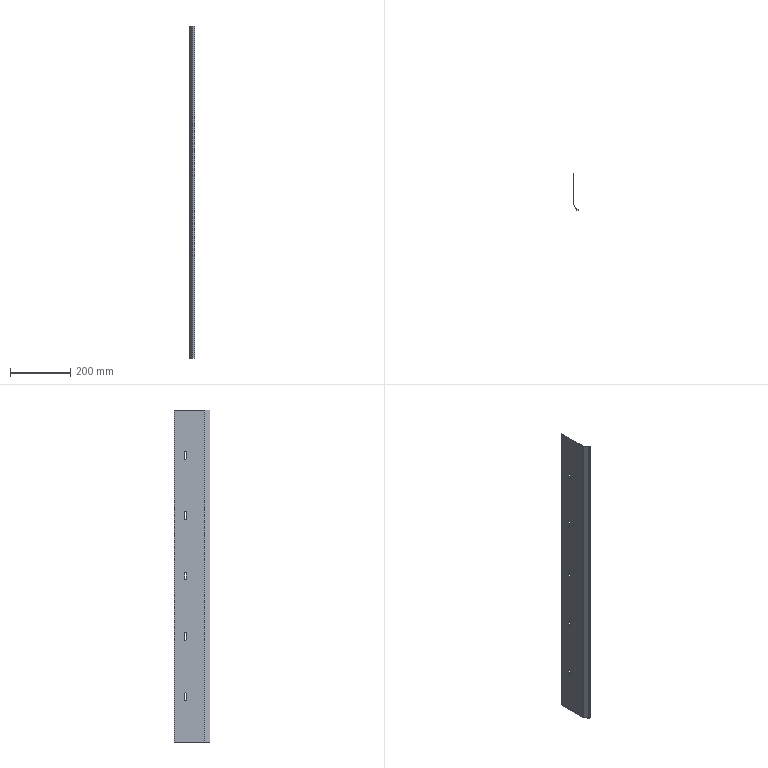Part | SolidWorks | features FlatPattern 1, ICE 1, SMBaseFlange 1, SheetMetal 1 | 1 solid | 47 faces | box 17 x 118.321 x 1100 mm | volume 138591 mm3 | plane 28 | cylinder 19 | commonest cylinder face diameters 6 x15 2 x2 4 x2
STEP:
#1=CARTESIAN_POINT('',(0.,-34.5,210.));
#2=VERTEX_POINT('',#1);
#3=CARTESIAN_POINT('',(0.,-37.5,213.));
#4=VERTEX_POINT('',#3);
#5=CARTESIAN_POINT('',(0.,-37.5,210.));
#6=DIRECTION('',(1.,0.,0.));
#7=DIRECTION('',(0.,1.,0.));
#8=AXIS2_PLACEMENT_3D('',#5,#6,#7);
#9=CIRCLE('',#8,3.);
#10=EDGE_CURVE('',#2,#4,#9,.T.);
#11=ORIENTED_EDGE('',*,*,#10,.T.);
#12=CARTESIAN_POINT('',(-1.,-37.5,213.));
#13=VERTEX_POINT('',#12);
#14=CARTESIAN_POINT('',(9.,-37.5,213.));
#15=DIRECTION('',(-1.,0.,0.));
#16=VECTOR('',#15,1000.);
#17=LINE('',#14,#16);
#18=EDGE_CURVE('',#4,#13,#17,.T.);
#19=ORIENTED_EDGE('',*,*,#18,.T.);
#20=CARTESIAN_POINT('',(-1.,-34.5,210.));
#21=VERTEX_POINT('',#20);
#22=CARTESIAN_POINT('',(-1.,-37.5,210.));
#23=DIRECTION('',(-1.,0.,0.));
#24=DIRECTION('',(0.,0.,-1.));
#25=AXIS2_PLACEMENT_3D('',#22,#23,#24);
#26=CIRCLE('',#25,3.);
#27=EDGE_CURVE('',#13,#21,#26,.T.);
#28=ORIENTED_EDGE('',*,*,#27,.T.);
#29=CARTESIAN_POINT('',(9.,-34.5,210.));
#30=DIRECTION('',(-1.,0.,0.));
#31=VECTOR('',#30,1000.);
#32=LINE('',#29,#31);
#33=EDGE_CURVE('',#2,#21,#32,.T.);
#34=ORIENTED_EDGE('',*,*,#33,.F.);
#35=EDGE_LOOP('',(#11,#19,#28,#34));
#36=FACE_OUTER_BOUND('',#35,.T.);
#37=CARTESIAN_POINT('',(9.,-37.5,210.));
#38=DIRECTION('',(-1.,0.,0.));
#39=DIRECTION('',(0.,0.,1.));
#40=AXIS2_PLACEMENT_3D('',#37,#38,#39);
#41=CYLINDRICAL_SURFACE('',#40,3.);
#42=ADVANCED_FACE('',(#36),#41,.F.);
#43=CARTESIAN_POINT('',(0.,-34.5,410.));
#44=VERTEX_POINT('',#43);
#45=CARTESIAN_POINT('',(0.,-37.5,413.));
#46=VERTEX_POINT('',#45);
#47=CARTESIAN_POINT('',(0.,-37.5,410.));
#48=DIRECTION('',(1.,0.,0.));
#49=DIRECTION('',(0.,1.,0.));
#50=AXIS2_PLACEMENT_3D('',#47,#48,#49);
#51=CIRCLE('',#50,3.);
#52=EDGE_CURVE('',#44,#46,#51,.T.);
#53=ORIENTED_EDGE('',*,*,#52,.T.);
#54=CARTESIAN_POINT('',(-1.,-37.5,413.));
#55=VERTEX_POINT('',#54);
#56=CARTESIAN_POINT('',(9.,-37.5,413.));
#57=DIRECTION('',(-1.,0.,0.));
#58=VECTOR('',#57,1000.);
#59=LINE('',#56,#58);
#60=EDGE_CURVE('',#46,#55,#59,.T.);
#61=ORIENTED_EDGE('',*,*,#60,.T.);
#62=CARTESIAN_POINT('',(-1.,-34.5,410.));
#63=VERTEX_POINT('',#62);
#64=CARTESIAN_POINT('',(-1.,-37.5,410.));
#65=DIRECTION('',(-1.,0.,0.));
#66=DIRECTION('',(0.,0.,-1.));
#67=AXIS2_PLACEMENT_3D('',#64,#65,#66);
#68=CIRCLE('',#67,3.);
#69=EDGE_CURVE('',#55,#63,#68,.T.);
#70=ORIENTED_EDGE('',*,*,#69,.T.);
#71=CARTESIAN_POINT('',(9.,-34.5,410.));
#72=DIRECTION('',(-1.,0.,0.));
#73=VECTOR('',#72,1000.);
#74=LINE('',#71,#73);
#75=EDGE_CURVE('',#44,#63,#74,.T.);
#76=ORIENTED_EDGE('',*,*,#75,.F.);
#77=EDGE_LOOP('',(#53,#61,#70,#76));
#78=FACE_OUTER_BOUND('',#77,.T.);
#79=CARTESIAN_POINT('',(9.,-37.5,410.));
#80=DIRECTION('',(-1.,0.,0.));
#81=DIRECTION('',(0.,0.,1.));
#82=AXIS2_PLACEMENT_3D('',#79,#80,#81);
#83=CYLINDRICAL_SURFACE('',#82,3.);
#84=ADVANCED_FACE('',(#78),#83,.F.);
#85=CARTESIAN_POINT('',(0.,-34.5,-390.));
#86=VERTEX_POINT('',#85);
#87=CARTESIAN_POINT('',(0.,-37.5,-387.));
#88=VERTEX_POINT('',#87);
#89=CARTESIAN_POINT('',(0.,-37.5,-390.));
#90=DIRECTION('',(1.,0.,0.));
#91=DIRECTION('',(0.,1.,0.));
#92=AXIS2_PLACEMENT_3D('',#89,#90,#91);
#93=CIRCLE('',#92,3.);
#94=EDGE_CURVE('',#86,#88,#93,.T.);
#95=ORIENTED_EDGE('',*,*,#94,.T.);
#96=CARTESIAN_POINT('',(-1.,-37.5,-387.));
#97=VERTEX_POINT('',#96);
#98=CARTESIAN_POINT('',(9.,-37.5,-387.));
#99=DIRECTION('',(-1.,0.,0.));
#100=VECTOR('',#99,1000.);
#101=LINE('',#98,#100);
#102=EDGE_CURVE('',#88,#97,#101,.T.);
#103=ORIENTED_EDGE('',*,*,#102,.T.);
#104=CARTESIAN_POINT('',(-1.,-34.5,-390.));
#105=VERTEX_POINT('',#104);
#106=CARTESIAN_POINT('',(-1.,-37.5,-390.));
#107=DIRECTION('',(-1.,0.,0.));
#108=DIRECTION('',(0.,0.,1.));
#109=AXIS2_PLACEMENT_3D('',#106,#107,#108);
#110=CIRCLE('',#109,3.);
#111=EDGE_CURVE('',#97,#105,#110,.T.);
#112=ORIENTED_EDGE('',*,*,#111,.T.);
#113=CARTESIAN_POINT('',(9.,-34.5,-390.));
#114=DIRECTION('',(-1.,0.,0.));
#115=VECTOR('',#114,1000.);
#116=LINE('',#113,#115);
#117=EDGE_CURVE('',#86,#105,#116,.T.);
#118=ORIENTED_EDGE('',*,*,#117,.F.);
#119=EDGE_LOOP('',(#95,#103,#112,#118));
#120=FACE_OUTER_BOUND('',#119,.T.);
#121=CARTESIAN_POINT('',(9.,-37.5,-390.));
#122=DIRECTION('',(-1.,0.,0.));
#123=DIRECTION('',(0.,0.,1.));
#124=AXIS2_PLACEMENT_3D('',#121,#122,#123);
#125=CYLINDRICAL_SURFACE('',#124,3.);
#126=ADVANCED_FACE('',(#120),#125,.F.);
#127=CARTESIAN_POINT('',(0.,-34.5,-190.));
#128=VERTEX_POINT('',#127);
#129=CARTESIAN_POINT('',(0.,-37.5,-187.));
#130=VERTEX_POINT('',#129);
#131=CARTESIAN_POINT('',(0.,-37.5,-190.));
#132=DIRECTION('',(1.,0.,0.));
#133=DIRECTION('',(0.,1.,0.));
#134=AXIS2_PLACEMENT_3D('',#131,#132,#133);
#135=CIRCLE('',#134,3.);
#136=EDGE_CURVE('',#128,#130,#135,.T.);
#137=ORIENTED_EDGE('',*,*,#136,.T.);
#138=CARTESIAN_POINT('',(-1.,-37.5,-187.));
#139=VERTEX_POINT('',#138);
#140=CARTESIAN_POINT('',(9.,-37.5,-187.));
#141=DIRECTION('',(-1.,0.,0.));
#142=VECTOR('',#141,1000.);
#143=LINE('',#140,#142);
#144=EDGE_CURVE('',#130,#139,#143,.T.);
#145=ORIENTED_EDGE('',*,*,#144,.T.);
#146=CARTESIAN_POINT('',(-1.,-34.5,-190.));
#147=VERTEX_POINT('',#146);
#148=CARTESIAN_POINT('',(-1.,-37.5,-190.));
#149=DIRECTION('',(-1.,0.,0.));
#150=DIRECTION('',(0.,0.,1.));
#151=AXIS2_PLACEMENT_3D('',#148,#149,#150);
#152=CIRCLE('',#151,3.);
#153=EDGE_CURVE('',#139,#147,#152,.T.);
#154=ORIENTED_EDGE('',*,*,#153,.T.);
#155=CARTESIAN_POINT('',(9.,-34.5,-190.));
#156=DIRECTION('',(-1.,0.,0.));
#157=VECTOR('',#156,1000.);
#158=LINE('',#155,#157);
#159=EDGE_CURVE('',#128,#147,#158,.T.);
#160=ORIENTED_EDGE('',*,*,#159,.F.);
#161=EDGE_LOOP('',(#137,#145,#154,#160));
#162=FACE_OUTER_BOUND('',#161,.T.);
#163=CARTESIAN_POINT('',(9.,-37.5,-190.));
#164=DIRECTION('',(-1.,0.,0.));
#165=DIRECTION('',(0.,0.,1.));
#166=AXIS2_PLACEMENT_3D('',#163,#164,#165);
#167=CYLINDRICAL_SURFACE('',#166,3.);
#168=ADVANCED_FACE('',(#162),#167,.F.);
#169=CARTESIAN_POINT('',(0.,-34.5,10.));
#170=VERTEX_POINT('',#169);
#171=CARTESIAN_POINT('',(0.,-37.5,13.));
#172=VERTEX_POINT('',#171);
#173=CARTESIAN_POINT('',(0.,-37.5,10.));
#174=DIRECTION('',(1.,0.,0.));
#175=DIRECTION('',(0.,1.,0.));
#176=AXIS2_PLACEMENT_3D('',#173,#174,#175);
#177=CIRCLE('',#176,3.);
#178=EDGE_CURVE('',#170,#172,#177,.T.);
#179=ORIENTED_EDGE('',*,*,#178,.T.);
#180=CARTESIAN_POINT('',(-1.,-37.5,13.));
#181=VERTEX_POINT('',#180);
#182=CARTESIAN_POINT('',(9.,-37.5,13.));
#183=DIRECTION('',(-1.,0.,0.));
#184=VECTOR('',#183,1000.);
#185=LINE('',#182,#184);
#186=EDGE_CURVE('',#172,#181,#185,.T.);
#187=ORIENTED_EDGE('',*,*,#186,.T.);
#188=CARTESIAN_POINT('',(-1.,-34.5,10.));
#189=VERTEX_POINT('',#188);
#190=CARTESIAN_POINT('',(-1.,-37.5,10.));
#191=DIRECTION('',(-1.,0.,0.));
#192=DIRECTION('',(0.,0.,1.));
#193=AXIS2_PLACEMENT_3D('',#190,#191,#192);
#194=CIRCLE('',#193,3.);
#195=EDGE_CURVE('',#181,#189,#194,.T.);
#196=ORIENTED_EDGE('',*,*,#195,.T.);
#197=CARTESIAN_POINT('',(9.,-34.5,10.));
#198=DIRECTION('',(-1.,0.,0.));
#199=VECTOR('',#198,1000.);
#200=LINE('',#197,#199);
#201=EDGE_CURVE('',#170,#189,#200,.T.);
#202=ORIENTED_EDGE('',*,*,#201,.F.);
#203=EDGE_LOOP('',(#179,#187,#196,#202));
#204=FACE_OUTER_BOUND('',#203,.T.);
#205=CARTESIAN_POINT('',(9.,-37.5,10.));
#206=DIRECTION('',(-1.,0.,0.));
#207=DIRECTION('',(0.,0.,1.));
#208=AXIS2_PLACEMENT_3D('',#205,#206,#207);
#209=CYLINDRICAL_SURFACE('',#208,3.);
#210=ADVANCED_FACE('',(#204),#209,.F.);
#211=CARTESIAN_POINT('',(0.134,-100.232,550.));
#212=VERTEX_POINT('',#211);
#213=CARTESIAN_POINT('',(-0.7321,-100.732,550.));
#214=VERTEX_POINT('',#213);
#215=CARTESIAN_POINT('',(0.134,-100.232,550.));
#216=DIRECTION('',(-0.866,-0.5,0.));
#217=VECTOR('',#216,1000.);
#218=LINE('',#215,#217);
#219=EDGE_CURVE('',#212,#214,#218,.T.);
#220=ORIENTED_EDGE('',*,*,#219,.F.);
#221=CARTESIAN_POINT('',(0.,-99.732,550.));
#222=VERTEX_POINT('',#221);
#223=CARTESIAN_POINT('',(1.,-99.732,550.));
#224=DIRECTION('',(0.,0.,1.));
#225=DIRECTION('',(-1.,0.,0.));
#226=AXIS2_PLACEMENT_3D('',#223,#224,#225);
#227=CIRCLE('',#226,1.);
#228=EDGE_CURVE('',#222,#212,#227,.T.);
#229=ORIENTED_EDGE('',*,*,#228,.F.);
#230=CARTESIAN_POINT('',(-1.,-99.732,550.));
#231=VERTEX_POINT('',#230);
#232=CARTESIAN_POINT('',(-1.,-99.732,550.));
#233=DIRECTION('',(1.,0.,0.));
#234=VECTOR('',#233,1000.);
#235=LINE('',#232,#234);
#236=EDGE_CURVE('',#231,#222,#235,.T.);
#237=ORIENTED_EDGE('',*,*,#236,.F.);
#238=CARTESIAN_POINT('',(1.,-99.732,550.));
#239=DIRECTION('',(0.,0.,1.));
#240=DIRECTION('',(1.,0.,0.));
#241=AXIS2_PLACEMENT_3D('',#238,#239,#240);
#242=CIRCLE('',#241,2.);
#243=EDGE_CURVE('',#231,#214,#242,.T.);
#244=ORIENTED_EDGE('',*,*,#243,.T.);
#245=EDGE_LOOP('',(#220,#229,#237,#244));
#246=FACE_OUTER_BOUND('',#245,.T.);
#247=CARTESIAN_POINT('',(0.134,-100.232,550.));
#248=DIRECTION('',(0.,0.,1.));
#249=DIRECTION('',(1.,0.,0.));
#250=AXIS2_PLACEMENT_3D('',#247,#248,#249);
#251=PLANE('',#250);
#252=ADVANCED_FACE('',(#246),#251,.T.);
#253=CARTESIAN_POINT('',(9.711,-116.821,550.));
#254=VERTEX_POINT('',#253);
#255=CARTESIAN_POINT('',(0.,-100.,550.));
#256=DIRECTION('',(0.5,-0.866,0.));
#257=VECTOR('',#256,1000.);
#258=LINE('',#255,#257);
#259=EDGE_CURVE('',#212,#254,#258,.T.);
#260=ORIENTED_EDGE('',*,*,#259,.F.);
#261=ORIENTED_EDGE('',*,*,#219,.T.);
#262=CARTESIAN_POINT('',(8.845,-117.321,550.));
#263=VERTEX_POINT('',#262);
#264=CARTESIAN_POINT('',(-0.866,-100.5,550.));
#265=DIRECTION('',(0.5,-0.866,0.));
#266=VECTOR('',#265,1000.);
#267=LINE('',#264,#266);
#268=EDGE_CURVE('',#214,#263,#267,.T.);
#269=ORIENTED_EDGE('',*,*,#268,.T.);
#270=CARTESIAN_POINT('',(8.845,-117.321,550.));
#271=DIRECTION('',(0.866,0.5,0.));
#272=VECTOR('',#271,1000.);
#273=LINE('',#270,#272);
#274=EDGE_CURVE('',#263,#254,#273,.T.);
#275=ORIENTED_EDGE('',*,*,#274,.T.);
#276=EDGE_LOOP('',(#260,#261,#269,#275));
#277=FACE_OUTER_BOUND('',#276,.T.);
#278=CARTESIAN_POINT('',(-1.,-99.732,550.));
#279=DIRECTION('',(0.,0.,1.));
#280=DIRECTION('',(1.,0.,0.));
#281=AXIS2_PLACEMENT_3D('',#278,#279,#280);
#282=PLANE('',#281);
#283=ADVANCED_FACE('',(#277),#282,.T.);
#284=CARTESIAN_POINT('',(0.,-99.732,-550.));
#285=VERTEX_POINT('',#284);
#286=CARTESIAN_POINT('',(-1.,-99.732,-550.));
#287=VERTEX_POINT('',#286);
#288=CARTESIAN_POINT('',(0.,-99.732,-550.));
#289=DIRECTION('',(-1.,0.,0.));
#290=VECTOR('',#289,1000.);
#291=LINE('',#288,#290);
#292=EDGE_CURVE('',#285,#287,#291,.T.);
#293=ORIENTED_EDGE('',*,*,#292,.F.);
#294=CARTESIAN_POINT('',(0.134,-100.232,-550.));
#295=VERTEX_POINT('',#294);
#296=CARTESIAN_POINT('',(1.,-99.732,-550.));
#297=DIRECTION('',(0.,0.,1.));
#298=DIRECTION('',(-1.,0.,0.));
#299=AXIS2_PLACEMENT_3D('',#296,#297,#298);
#300=CIRCLE('',#299,1.);
#301=EDGE_CURVE('',#285,#295,#300,.T.);
#302=ORIENTED_EDGE('',*,*,#301,.T.);
#303=CARTESIAN_POINT('',(-0.7321,-100.732,-550.));
#304=VERTEX_POINT('',#303);
#305=CARTESIAN_POINT('',(-0.7321,-100.732,-550.));
#306=DIRECTION('',(0.866,0.5,0.));
#307=VECTOR('',#306,1000.);
#308=LINE('',#305,#307);
#309=EDGE_CURVE('',#304,#295,#308,.T.);
#310=ORIENTED_EDGE('',*,*,#309,.F.);
#311=CARTESIAN_POINT('',(1.,-99.732,-550.));
#312=DIRECTION('',(0.,0.,1.));
#313=DIRECTION('',(1.,0.,0.));
#314=AXIS2_PLACEMENT_3D('',#311,#312,#313);
#315=CIRCLE('',#314,2.);
#316=EDGE_CURVE('',#287,#304,#315,.T.);
#317=ORIENTED_EDGE('',*,*,#316,.F.);
#318=EDGE_LOOP('',(#293,#302,#310,#317));
#319=FACE_OUTER_BOUND('',#318,.T.);
#320=CARTESIAN_POINT('',(0.,-99.732,-550.));
#321=DIRECTION('',(0.,0.,-1.));
#322=DIRECTION('',(-1.,0.,0.));
#323=AXIS2_PLACEMENT_3D('',#320,#321,#322);
#324=PLANE('',#323);
#325=ADVANCED_FACE('',(#319),#324,.T.);
#326=CARTESIAN_POINT('',(0.,0.,-550.));
#327=VERTEX_POINT('',#326);
#328=CARTESIAN_POINT('',(0.,0.,-550.));
#329=DIRECTION('',(0.,-1.,0.));
#330=VECTOR('',#329,1000.);
#331=LINE('',#328,#330);
#332=EDGE_CURVE('',#327,#285,#331,.T.);
#333=ORIENTED_EDGE('',*,*,#332,.T.);
#334=ORIENTED_EDGE('',*,*,#292,.T.);
#335=CARTESIAN_POINT('',(-1.,0.,-550.));
#336=VERTEX_POINT('',#335);
#337=CARTESIAN_POINT('',(-1.,0.,-550.));
#338=DIRECTION('',(0.,-1.,0.));
#339=VECTOR('',#338,1000.);
#340=LINE('',#337,#339);
#341=EDGE_CURVE('',#336,#287,#340,.T.);
#342=ORIENTED_EDGE('',*,*,#341,.F.);
#343=CARTESIAN_POINT('',(-1.,0.,-550.));
#344=DIRECTION('',(1.,0.,0.));
#345=VECTOR('',#344,1000.);
#346=LINE('',#343,#345);
#347=EDGE_CURVE('',#336,#327,#346,.T.);
#348=ORIENTED_EDGE('',*,*,#347,.T.);
#349=EDGE_LOOP('',(#333,#334,#342,#348));
#350=FACE_OUTER_BOUND('',#349,.T.);
#351=CARTESIAN_POINT('',(-0.7321,-100.732,-550.));
#352=DIRECTION('',(0.,0.,-1.));
#353=DIRECTION('',(-1.,0.,0.));
#354=AXIS2_PLACEMENT_3D('',#351,#352,#353);
#355=PLANE('',#354);
#356=ADVANCED_FACE('',(#350),#355,.T.);
#357=CARTESIAN_POINT('',(10.577,-117.321,550.));
#358=VERTEX_POINT('',#357);
#359=CARTESIAN_POINT('',(10.577,-118.321,550.));
#360=VERTEX_POINT('',#359);
#361=CARTESIAN_POINT('',(10.577,-117.321,550.));
#362=DIRECTION('',(0.,-1.,0.));
#363=VECTOR('',#362,1000.);
#364=LINE('',#361,#363);
#365=EDGE_CURVE('',#358,#360,#364,.T.);
#366=ORIENTED_EDGE('',*,*,#365,.F.);
#367=CARTESIAN_POINT('',(10.577,-116.321,550.));
#368=DIRECTION('',(0.,0.,1.));
#369=DIRECTION('',(-1.,0.,0.));
#370=AXIS2_PLACEMENT_3D('',#367,#368,#369);
#371=CIRCLE('',#370,1.);
#372=EDGE_CURVE('',#254,#358,#371,.T.);
#373=ORIENTED_EDGE('',*,*,#372,.F.);
#374=ORIENTED_EDGE('',*,*,#274,.F.);
#375=CARTESIAN_POINT('',(10.577,-116.321,550.));
#376=DIRECTION('',(0.,0.,1.));
#377=DIRECTION('',(1.,0.,0.));
#378=AXIS2_PLACEMENT_3D('',#375,#376,#377);
#379=CIRCLE('',#378,2.);
#380=EDGE_CURVE('',#263,#360,#379,.T.);
#381=ORIENTED_EDGE('',*,*,#380,.T.);
#382=EDGE_LOOP('',(#366,#373,#374,#381));
#383=FACE_OUTER_BOUND('',#382,.T.);
#384=CARTESIAN_POINT('',(10.577,-117.321,550.));
#385=DIRECTION('',(0.,0.,1.));
#386=DIRECTION('',(1.,0.,0.));
#387=AXIS2_PLACEMENT_3D('',#384,#385,#386);
#388=PLANE('',#387);
#389=ADVANCED_FACE('',(#383),#388,.T.);
#390=CARTESIAN_POINT('',(16.,-117.321,550.));
#391=VERTEX_POINT('',#390);
#392=CARTESIAN_POINT('',(10.,-117.321,550.));
#393=DIRECTION('',(1.,0.,0.));
#394=VECTOR('',#393,1000.);
#395=LINE('',#392,#394);
#396=EDGE_CURVE('',#358,#391,#395,.T.);
#397=ORIENTED_EDGE('',*,*,#396,.F.);
#398=ORIENTED_EDGE('',*,*,#365,.T.);
#399=CARTESIAN_POINT('',(16.,-118.321,550.));
#400=VERTEX_POINT('',#399);
#401=CARTESIAN_POINT('',(10.,-118.321,550.));
#402=DIRECTION('',(1.,0.,0.));
#403=VECTOR('',#402,1000.);
#404=LINE('',#401,#403);
#405=EDGE_CURVE('',#360,#400,#404,.T.);
#406=ORIENTED_EDGE('',*,*,#405,.T.);
#407=CARTESIAN_POINT('',(16.,-117.321,550.));
#408=DIRECTION('',(0.,-1.,0.));
#409=VECTOR('',#408,1000.);
#410=LINE('',#407,#409);
#411=EDGE_CURVE('',#391,#400,#410,.T.);
#412=ORIENTED_EDGE('',*,*,#411,.F.);
#413=EDGE_LOOP('',(#397,#398,#406,#412));
#414=FACE_OUTER_BOUND('',#413,.T.);
#415=CARTESIAN_POINT('',(8.845,-117.321,550.));
#416=DIRECTION('',(0.,0.,1.));
#417=DIRECTION('',(1.,0.,0.));
#418=AXIS2_PLACEMENT_3D('',#415,#416,#417);
#419=PLANE('',#418);
#420=ADVANCED_FACE('',(#414),#419,.T.);
#421=CARTESIAN_POINT('',(9.711,-116.821,-550.));
#422=VERTEX_POINT('',#421);
#423=CARTESIAN_POINT('',(8.845,-117.321,-550.));
#424=VERTEX_POINT('',#423);
#425=CARTESIAN_POINT('',(9.711,-116.821,-550.));
#426=DIRECTION('',(-0.866,-0.5,0.));
#427=VECTOR('',#426,1000.);
#428=LINE('',#425,#427);
#429=EDGE_CURVE('',#422,#424,#428,.T.);
#430=ORIENTED_EDGE('',*,*,#429,.F.);
#431=CARTESIAN_POINT('',(10.577,-117.321,-550.));
#432=VERTEX_POINT('',#431);
#433=CARTESIAN_POINT('',(10.577,-116.321,-550.));
#434=DIRECTION('',(0.,0.,1.));
#435=DIRECTION('',(-1.,0.,0.));
#436=AXIS2_PLACEMENT_3D('',#433,#434,#435);
#437=CIRCLE('',#436,1.);
#438=EDGE_CURVE('',#422,#432,#437,.T.);
#439=ORIENTED_EDGE('',*,*,#438,.T.);
#440=CARTESIAN_POINT('',(10.577,-118.321,-550.));
#441=VERTEX_POINT('',#440);
#442=CARTESIAN_POINT('',(10.577,-118.321,-550.));
#443=DIRECTION('',(0.,1.,0.));
#444=VECTOR('',#443,1000.);
#445=LINE('',#442,#444);
#446=EDGE_CURVE('',#441,#432,#445,.T.);
#447=ORIENTED_EDGE('',*,*,#446,.F.);
#448=CARTESIAN_POINT('',(10.577,-116.321,-550.));
#449=DIRECTION('',(0.,0.,1.));
#450=DIRECTION('',(1.,0.,0.));
#451=AXIS2_PLACEMENT_3D('',#448,#449,#450);
#452=CIRCLE('',#451,2.);
#453=EDGE_CURVE('',#424,#441,#452,.T.);
#454=ORIENTED_EDGE('',*,*,#453,.F.);
#455=EDGE_LOOP('',(#430,#439,#447,#454));
#456=FACE_OUTER_BOUND('',#455,.T.);
#457=CARTESIAN_POINT('',(9.711,-116.821,-550.));
#458=DIRECTION('',(0.,0.,-1.));
#459=DIRECTION('',(-1.,0.,0.));
#460=AXIS2_PLACEMENT_3D('',#457,#458,#459);
#461=PLANE('',#460);
#462=ADVANCED_FACE('',(#456),#461,.T.);
#463=CARTESIAN_POINT('',(0.,-100.,-550.));
#464=DIRECTION('',(0.5,-0.866,0.));
#465=VECTOR('',#464,1000.);
#466=LINE('',#463,#465);
#467=EDGE_CURVE('',#295,#422,#466,.T.);
#468=ORIENTED_EDGE('',*,*,#467,.T.);
#469=ORIENTED_EDGE('',*,*,#429,.T.);
#470=CARTESIAN_POINT('',(-0.866,-100.5,-550.));
#471=DIRECTION('',(0.5,-0.866,0.));
#472=VECTOR('',#471,1000.);
#473=LINE('',#470,#472);
#474=EDGE_CURVE('',#304,#424,#473,.T.);
#475=ORIENTED_EDGE('',*,*,#474,.F.);
#476=ORIENTED_EDGE('',*,*,#309,.T.);
#477=EDGE_LOOP('',(#468,#469,#475,#476));
#478=FACE_OUTER_BOUND('',#477,.T.);
#479=CARTESIAN_POINT('',(10.577,-118.321,-550.));
#480=DIRECTION('',(0.,0.,-1.));
#481=DIRECTION('',(-1.,0.,0.));
#482=AXIS2_PLACEMENT_3D('',#479,#480,#481);
#483=PLANE('',#482);
#484=ADVANCED_FACE('',(#478),#483,.T.);
#485=CARTESIAN_POINT('',(16.,-118.321,-550.));
#486=VERTEX_POINT('',#485);
#487=CARTESIAN_POINT('',(10.,-118.321,-550.));
#488=DIRECTION('',(1.,0.,0.));
#489=VECTOR('',#488,1000.);
#490=LINE('',#487,#489);
#491=EDGE_CURVE('',#441,#486,#490,.T.);
#492=ORIENTED_EDGE('',*,*,#491,.T.);
#493=CARTESIAN_POINT('',(16.,-118.321,550.));
#494=DIRECTION('',(0.,0.,-1.));
#495=VECTOR('',#494,1000.);
#496=LINE('',#493,#495);
#497=EDGE_CURVE('',#400,#486,#496,.T.);
#498=ORIENTED_EDGE('',*,*,#497,.F.);
#499=ORIENTED_EDGE('',*,*,#405,.F.);
#500=CARTESIAN_POINT('',(10.577,-118.321,550.));
#501=DIRECTION('',(0.,0.,-1.));
#502=VECTOR('',#501,1000.);
#503=LINE('',#500,#502);
#504=EDGE_CURVE('',#360,#441,#503,.T.);
#505=ORIENTED_EDGE('',*,*,#504,.T.);
#506=EDGE_LOOP('',(#492,#498,#499,#505));
#507=FACE_OUTER_BOUND('',#506,.T.);
#508=CARTESIAN_POINT('',(10.,-118.321,550.));
#509=DIRECTION('',(0.,1.,0.));
#510=DIRECTION('',(0.,0.,1.));
#511=AXIS2_PLACEMENT_3D('',#508,#509,#510);
#512=PLANE('',#511);
#513=ADVANCED_FACE('',(#507),#512,.F.);
#514=CARTESIAN_POINT('',(16.,-117.321,-550.));
#515=VERTEX_POINT('',#514);
#516=CARTESIAN_POINT('',(16.,-117.321,-550.));
#517=DIRECTION('',(0.,-1.,0.));
#518=VECTOR('',#517,1000.);
#519=LINE('',#516,#518);
#520=EDGE_CURVE('',#515,#486,#519,.T.);
#521=ORIENTED_EDGE('',*,*,#520,.F.);
#522=CARTESIAN_POINT('',(16.,-117.321,550.));
#523=DIRECTION('',(0.,0.,-1.));
#524=VECTOR('',#523,1000.);
#525=LINE('',#522,#524);
#526=EDGE_CURVE('',#391,#515,#525,.T.);
#527=ORIENTED_EDGE('',*,*,#526,.F.);
#528=ORIENTED_EDGE('',*,*,#411,.T.);
#529=ORIENTED_EDGE('',*,*,#497,.T.);
#530=EDGE_LOOP('',(#521,#527,#528,#529));
#531=FACE_OUTER_BOUND('',#530,.T.);
#532=CARTESIAN_POINT('',(16.,-117.321,550.));
#533=DIRECTION('',(1.,0.,0.));
#534=DIRECTION('',(0.,0.,-1.));
#535=AXIS2_PLACEMENT_3D('',#532,#533,#534);
#536=PLANE('',#535);
#537=ADVANCED_FACE('',(#531),#536,.T.);
#538=CARTESIAN_POINT('',(10.,-117.321,-550.));
#539=DIRECTION('',(1.,0.,0.));
#540=VECTOR('',#539,1000.);
#541=LINE('',#538,#540);
#542=EDGE_CURVE('',#432,#515,#541,.T.);
#543=ORIENTED_EDGE('',*,*,#542,.F.);
#544=CARTESIAN_POINT('',(10.577,-117.321,550.));
#545=DIRECTION('',(0.,0.,-1.));
#546=VECTOR('',#545,1000.);
#547=LINE('',#544,#546);
#548=EDGE_CURVE('',#358,#432,#547,.T.);
#549=ORIENTED_EDGE('',*,*,#548,.F.);
#550=ORIENTED_EDGE('',*,*,#396,.T.);
#551=ORIENTED_EDGE('',*,*,#526,.T.);
#552=EDGE_LOOP('',(#543,#549,#550,#551));
#553=FACE_OUTER_BOUND('',#552,.T.);
#554=CARTESIAN_POINT('',(10.,-117.321,550.));
#555=DIRECTION('',(0.,1.,0.));
#556=DIRECTION('',(0.,0.,1.));
#557=AXIS2_PLACEMENT_3D('',#554,#555,#556);
#558=PLANE('',#557);
#559=ADVANCED_FACE('',(#553),#558,.T.);
#560=ORIENTED_EDGE('',*,*,#438,.F.);
#561=CARTESIAN_POINT('',(9.711,-116.821,550.));
#562=DIRECTION('',(0.,0.,-1.));
#563=VECTOR('',#562,1000.);
#564=LINE('',#561,#563);
#565=EDGE_CURVE('',#254,#422,#564,.T.);
#566=ORIENTED_EDGE('',*,*,#565,.F.);
#567=ORIENTED_EDGE('',*,*,#372,.T.);
#568=ORIENTED_EDGE('',*,*,#548,.T.);
#569=EDGE_LOOP('',(#560,#566,#567,#568));
#570=FACE_OUTER_BOUND('',#569,.T.);
#571=CARTESIAN_POINT('',(10.577,-116.321,550.));
#572=DIRECTION('',(0.,0.,-1.));
#573=DIRECTION('',(-1.,0.,0.));
#574=AXIS2_PLACEMENT_3D('',#571,#572,#573);
#575=CYLINDRICAL_SURFACE('',#574,1.);
#576=ADVANCED_FACE('',(#570),#575,.F.);
#577=ORIENTED_EDGE('',*,*,#467,.F.);
#578=CARTESIAN_POINT('',(0.134,-100.232,550.));
#579=DIRECTION('',(0.,0.,-1.));
#580=VECTOR('',#579,1000.);
#581=LINE('',#578,#580);
#582=EDGE_CURVE('',#212,#295,#581,.T.);
#583=ORIENTED_EDGE('',*,*,#582,.F.);
#584=ORIENTED_EDGE('',*,*,#259,.T.);
#585=ORIENTED_EDGE('',*,*,#565,.T.);
#586=EDGE_LOOP('',(#577,#583,#584,#585));
#587=FACE_OUTER_BOUND('',#586,.T.);
#588=CARTESIAN_POINT('',(0.,-100.,550.));
#589=DIRECTION('',(0.866,0.5,0.));
#590=DIRECTION('',(-0.5,0.866,0.));
#591=AXIS2_PLACEMENT_3D('',#588,#589,#590);
#592=PLANE('',#591);
#593=ADVANCED_FACE('',(#587),#592,.T.);
#594=ORIENTED_EDGE('',*,*,#301,.F.);
#595=CARTESIAN_POINT('',(0.,-99.732,550.));
#596=DIRECTION('',(0.,0.,-1.));
#597=VECTOR('',#596,1000.);
#598=LINE('',#595,#597);
#599=EDGE_CURVE('',#222,#285,#598,.T.);
#600=ORIENTED_EDGE('',*,*,#599,.F.);
#601=ORIENTED_EDGE('',*,*,#228,.T.);
#602=ORIENTED_EDGE('',*,*,#582,.T.);
#603=EDGE_LOOP('',(#594,#600,#601,#602));
#604=FACE_OUTER_BOUND('',#603,.T.);
#605=CARTESIAN_POINT('',(1.,-99.732,550.));
#606=DIRECTION('',(0.,0.,-1.));
#607=DIRECTION('',(-1.,0.,0.));
#608=AXIS2_PLACEMENT_3D('',#605,#606,#607);
#609=CYLINDRICAL_SURFACE('',#608,1.);
#610=ADVANCED_FACE('',(#604),#609,.F.);
#611=ORIENTED_EDGE('',*,*,#10,.F.);
#612=CARTESIAN_POINT('',(0.,-34.5,190.));
#613=VERTEX_POINT('',#612);
#614=CARTESIAN_POINT('',(0.,-34.5,550.));
#615=DIRECTION('',(0.,0.,1.));
#616=VECTOR('',#615,1000.);
#617=LINE('',#614,#616);
#618=EDGE_CURVE('',#613,#2,#617,.T.);
#619=ORIENTED_EDGE('',*,*,#618,.F.);
#620=CARTESIAN_POINT('',(0.,-40.5,190.));
#621=VERTEX_POINT('',#620);
#622=CARTESIAN_POINT('',(0.,-37.5,190.));
#623=DIRECTION('',(1.,0.,0.));
#624=DIRECTION('',(0.,1.,0.));
#625=AXIS2_PLACEMENT_3D('',#622,#623,#624);
#626=CIRCLE('',#625,3.);
#627=EDGE_CURVE('',#621,#613,#626,.T.);
#628=ORIENTED_EDGE('',*,*,#627,.F.);
#629=CARTESIAN_POINT('',(0.,-40.5,210.));
#630=VERTEX_POINT('',#629);
#631=CARTESIAN_POINT('',(0.,-40.5,550.));
#632=DIRECTION('',(0.,0.,-1.));
#633=VECTOR('',#632,1000.);
#634=LINE('',#631,#633);
#635=EDGE_CURVE('',#630,#621,#634,.T.);
#636=ORIENTED_EDGE('',*,*,#635,.F.);
#637=CARTESIAN_POINT('',(0.,-37.5,210.));
#638=DIRECTION('',(1.,0.,0.));
#639=DIRECTION('',(0.,1.,0.));
#640=AXIS2_PLACEMENT_3D('',#637,#638,#639);
#641=CIRCLE('',#640,3.);
#642=EDGE_CURVE('',#4,#630,#641,.T.);
#643=ORIENTED_EDGE('',*,*,#642,.F.);
#644=EDGE_LOOP('',(#611,#619,#628,#636,#643));
#645=FACE_BOUND('',#644,.T.);
#646=ORIENTED_EDGE('',*,*,#52,.F.);
#647=CARTESIAN_POINT('',(0.,-34.5,390.));
#648=VERTEX_POINT('',#647);
#649=CARTESIAN_POINT('',(0.,-34.5,550.));
#650=DIRECTION('',(0.,0.,1.));
#651=VECTOR('',#650,1000.);
#652=LINE('',#649,#651);
#653=EDGE_CURVE('',#648,#44,#652,.T.);
#654=ORIENTED_EDGE('',*,*,#653,.F.);
#655=CARTESIAN_POINT('',(0.,-40.5,390.));
#656=VERTEX_POINT('',#655);
#657=CARTESIAN_POINT('',(0.,-37.5,390.));
#658=DIRECTION('',(1.,0.,0.));
#659=DIRECTION('',(0.,1.,0.));
#660=AXIS2_PLACEMENT_3D('',#657,#658,#659);
#661=CIRCLE('',#660,3.);
#662=EDGE_CURVE('',#656,#648,#661,.T.);
#663=ORIENTED_EDGE('',*,*,#662,.F.);
#664=CARTESIAN_POINT('',(0.,-40.5,410.));
#665=VERTEX_POINT('',#664);
#666=CARTESIAN_POINT('',(0.,-40.5,550.));
#667=DIRECTION('',(0.,0.,-1.));
#668=VECTOR('',#667,1000.);
#669=LINE('',#666,#668);
#670=EDGE_CURVE('',#665,#656,#669,.T.);
#671=ORIENTED_EDGE('',*,*,#670,.F.);
#672=CARTESIAN_POINT('',(0.,-37.5,410.));
#673=DIRECTION('',(1.,0.,0.));
#674=DIRECTION('',(0.,1.,0.));
#675=AXIS2_PLACEMENT_3D('',#672,#673,#674);
#676=CIRCLE('',#675,3.);
#677=EDGE_CURVE('',#46,#665,#676,.T.);
#678=ORIENTED_EDGE('',*,*,#677,.F.);
#679=EDGE_LOOP('',(#646,#654,#663,#671,#678));
#680=FACE_BOUND('',#679,.T.);
#681=CARTESIAN_POINT('',(0.,-40.5,-410.));
#682=VERTEX_POINT('',#681);
#683=CARTESIAN_POINT('',(0.,-34.5,-410.));
#684=VERTEX_POINT('',#683);
#685=CARTESIAN_POINT('',(0.,-37.5,-410.));
#686=DIRECTION('',(1.,0.,0.));
#687=DIRECTION('',(0.,1.,0.));
#688=AXIS2_PLACEMENT_3D('',#685,#686,#687);
#689=CIRCLE('',#688,3.);
#690=EDGE_CURVE('',#682,#684,#689,.T.);
#691=ORIENTED_EDGE('',*,*,#690,.F.);
#692=CARTESIAN_POINT('',(0.,-40.5,-390.));
#693=VERTEX_POINT('',#692);
#694=CARTESIAN_POINT('',(0.,-40.5,550.));
#695=DIRECTION('',(0.,0.,-1.));
#696=VECTOR('',#695,1000.);
#697=LINE('',#694,#696);
#698=EDGE_CURVE('',#693,#682,#697,.T.);
#699=ORIENTED_EDGE('',*,*,#698,.F.);
#700=CARTESIAN_POINT('',(0.,-37.5,-390.));
#701=DIRECTION('',(1.,0.,0.));
#702=DIRECTION('',(0.,1.,0.));
#703=AXIS2_PLACEMENT_3D('',#700,#701,#702);
#704=CIRCLE('',#703,3.);
#705=EDGE_CURVE('',#88,#693,#704,.T.);
#706=ORIENTED_EDGE('',*,*,#705,.F.);
#707=ORIENTED_EDGE('',*,*,#94,.F.);
#708=CARTESIAN_POINT('',(0.,-34.5,550.));
#709=DIRECTION('',(0.,0.,1.));
#710=VECTOR('',#709,1000.);
#711=LINE('',#708,#710);
#712=EDGE_CURVE('',#684,#86,#711,.T.);
#713=ORIENTED_EDGE('',*,*,#712,.F.);
#714=EDGE_LOOP('',(#691,#699,#706,#707,#713));
#715=FACE_BOUND('',#714,.T.);
#716=CARTESIAN_POINT('',(0.,-40.5,-210.));
#717=VERTEX_POINT('',#716);
#718=CARTESIAN_POINT('',(0.,-34.5,-210.));
#719=VERTEX_POINT('',#718);
#720=CARTESIAN_POINT('',(0.,-37.5,-210.));
#721=DIRECTION('',(1.,0.,0.));
#722=DIRECTION('',(0.,1.,0.));
#723=AXIS2_PLACEMENT_3D('',#720,#721,#722);
#724=CIRCLE('',#723,3.);
#725=EDGE_CURVE('',#717,#719,#724,.T.);
#726=ORIENTED_EDGE('',*,*,#725,.F.);
#727=CARTESIAN_POINT('',(0.,-40.5,-190.));
#728=VERTEX_POINT('',#727);
#729=CARTESIAN_POINT('',(0.,-40.5,550.));
#730=DIRECTION('',(0.,0.,-1.));
#731=VECTOR('',#730,1000.);
#732=LINE('',#729,#731);
#733=EDGE_CURVE('',#728,#717,#732,.T.);
#734=ORIENTED_EDGE('',*,*,#733,.F.);
#735=CARTESIAN_POINT('',(0.,-37.5,-190.));
#736=DIRECTION('',(1.,0.,0.));
#737=DIRECTION('',(0.,1.,0.));
#738=AXIS2_PLACEMENT_3D('',#735,#736,#737);
#739=CIRCLE('',#738,3.);
#740=EDGE_CURVE('',#130,#728,#739,.T.);
#741=ORIENTED_EDGE('',*,*,#740,.F.);
#742=ORIENTED_EDGE('',*,*,#136,.F.);
#743=CARTESIAN_POINT('',(0.,-34.5,550.));
#744=DIRECTION('',(0.,0.,1.));
#745=VECTOR('',#744,1000.);
#746=LINE('',#743,#745);
#747=EDGE_CURVE('',#719,#128,#746,.T.);
#748=ORIENTED_EDGE('',*,*,#747,.F.);
#749=EDGE_LOOP('',(#726,#734,#741,#742,#748));
#750=FACE_BOUND('',#749,.T.);
#751=CARTESIAN_POINT('',(0.,-40.5,-10.));
#752=VERTEX_POINT('',#751);
#753=CARTESIAN_POINT('',(0.,-34.5,-10.));
#754=VERTEX_POINT('',#753);
#755=CARTESIAN_POINT('',(0.,-37.5,-10.));
#756=DIRECTION('',(1.,0.,0.));
#757=DIRECTION('',(0.,1.,0.));
#758=AXIS2_PLACEMENT_3D('',#755,#756,#757);
#759=CIRCLE('',#758,3.);
#760=EDGE_CURVE('',#752,#754,#759,.T.);
#761=ORIENTED_EDGE('',*,*,#760,.F.);
#762=CARTESIAN_POINT('',(0.,-40.5,10.));
#763=VERTEX_POINT('',#762);
#764=CARTESIAN_POINT('',(0.,-40.5,550.));
#765=DIRECTION('',(0.,0.,-1.));
#766=VECTOR('',#765,1000.);
#767=LINE('',#764,#766);
#768=EDGE_CURVE('',#763,#752,#767,.T.);
#769=ORIENTED_EDGE('',*,*,#768,.F.);
#770=CARTESIAN_POINT('',(0.,-37.5,10.));
#771=DIRECTION('',(1.,0.,0.));
#772=DIRECTION('',(0.,1.,0.));
#773=AXIS2_PLACEMENT_3D('',#770,#771,#772);
#774=CIRCLE('',#773,3.);
#775=EDGE_CURVE('',#172,#763,#774,.T.);
#776=ORIENTED_EDGE('',*,*,#775,.F.);
#777=ORIENTED_EDGE('',*,*,#178,.F.);
#778=CARTESIAN_POINT('',(0.,-34.5,550.));
#779=DIRECTION('',(0.,0.,1.));
#780=VECTOR('',#779,1000.);
#781=LINE('',#778,#780);
#782=EDGE_CURVE('',#754,#170,#781,.T.);
#783=ORIENTED_EDGE('',*,*,#782,.F.);
#784=EDGE_LOOP('',(#761,#769,#776,#777,#783));
#785=FACE_BOUND('',#784,.T.);
#786=ORIENTED_EDGE('',*,*,#332,.F.);
#787=CARTESIAN_POINT('',(0.,0.,550.));
#788=VERTEX_POINT('',#787);
#789=CARTESIAN_POINT('',(0.,0.,550.));
#790=DIRECTION('',(0.,0.,-1.));
#791=VECTOR('',#790,1000.);
#792=LINE('',#789,#791);
#793=EDGE_CURVE('',#788,#327,#792,.T.);
#794=ORIENTED_EDGE('',*,*,#793,.F.);
#795=CARTESIAN_POINT('',(0.,0.,550.));
#796=DIRECTION('',(0.,-1.,0.));
#797=VECTOR('',#796,1000.);
#798=LINE('',#795,#797);
#799=EDGE_CURVE('',#788,#222,#798,.T.);
#800=ORIENTED_EDGE('',*,*,#799,.T.);
#801=ORIENTED_EDGE('',*,*,#599,.T.);
#802=EDGE_LOOP('',(#786,#794,#800,#801));
#803=FACE_OUTER_BOUND('',#802,.T.);
#804=CARTESIAN_POINT('',(0.,0.,550.));
#805=DIRECTION('',(1.,0.,0.));
#806=DIRECTION('',(0.,1.,0.));
#807=AXIS2_PLACEMENT_3D('',#804,#805,#806);
#808=PLANE('',#807);
#809=ADVANCED_FACE('',(#645,#680,#715,#750,#785,#803),#808,.T.);
#810=ORIENTED_EDGE('',*,*,#347,.F.);
#811=CARTESIAN_POINT('',(-1.,0.,550.));
#812=VERTEX_POINT('',#811);
#813=CARTESIAN_POINT('',(-1.,0.,550.));
#814=DIRECTION('',(0.,0.,-1.));
#815=VECTOR('',#814,1000.);
#816=LINE('',#813,#815);
#817=EDGE_CURVE('',#812,#336,#816,.T.);
#818=ORIENTED_EDGE('',*,*,#817,.F.);
#819=CARTESIAN_POINT('',(-1.,0.,550.));
#820=DIRECTION('',(1.,0.,0.));
#821=VECTOR('',#820,1000.);
#822=LINE('',#819,#821);
#823=EDGE_CURVE('',#812,#788,#822,.T.);
#824=ORIENTED_EDGE('',*,*,#823,.T.);
#825=ORIENTED_EDGE('',*,*,#793,.T.);
#826=EDGE_LOOP('',(#810,#818,#824,#825));
#827=FACE_OUTER_BOUND('',#826,.T.);
#828=CARTESIAN_POINT('',(-1.,0.,550.));
#829=DIRECTION('',(0.,1.,0.));
#830=DIRECTION('',(-1.,0.,0.));
#831=AXIS2_PLACEMENT_3D('',#828,#829,#830);
#832=PLANE('',#831);
#833=ADVANCED_FACE('',(#827),#832,.T.);
#834=CARTESIAN_POINT('',(-1.,-34.5,190.));
#835=VERTEX_POINT('',#834);
#836=CARTESIAN_POINT('',(-1.,-34.5,210.));
#837=DIRECTION('',(0.,0.,-1.));
#838=VECTOR('',#837,1000.);
#839=LINE('',#836,#838);
#840=EDGE_CURVE('',#21,#835,#839,.T.);
#841=ORIENTED_EDGE('',*,*,#840,.F.);
#842=ORIENTED_EDGE('',*,*,#27,.F.);
#843=CARTESIAN_POINT('',(-1.,-40.5,210.));
#844=VERTEX_POINT('',#843);
#845=CARTESIAN_POINT('',(-1.,-37.5,210.));
#846=DIRECTION('',(-1.,0.,0.));
#847=DIRECTION('',(0.,0.,-1.));
#848=AXIS2_PLACEMENT_3D('',#845,#846,#847);
#849=CIRCLE('',#848,3.);
#850=EDGE_CURVE('',#844,#13,#849,.T.);
#851=ORIENTED_EDGE('',*,*,#850,.F.);
#852=CARTESIAN_POINT('',(-1.,-40.5,190.));
#853=VERTEX_POINT('',#852);
#854=CARTESIAN_POINT('',(-1.,-40.5,210.));
#855=DIRECTION('',(0.,0.,1.));
#856=VECTOR('',#855,1000.);
#857=LINE('',#854,#856);
#858=EDGE_CURVE('',#853,#844,#857,.T.);
#859=ORIENTED_EDGE('',*,*,#858,.F.);
#860=CARTESIAN_POINT('',(-1.,-37.5,190.));
#861=DIRECTION('',(-1.,0.,0.));
#862=DIRECTION('',(0.,0.,-1.));
#863=AXIS2_PLACEMENT_3D('',#860,#861,#862);
#864=CIRCLE('',#863,3.);
#865=EDGE_CURVE('',#835,#853,#864,.T.);
#866=ORIENTED_EDGE('',*,*,#865,.F.);
#867=EDGE_LOOP('',(#841,#842,#851,#859,#866));
#868=FACE_BOUND('',#867,.T.);
#869=CARTESIAN_POINT('',(-1.,-34.5,390.));
#870=VERTEX_POINT('',#869);
#871=CARTESIAN_POINT('',(-1.,-34.5,410.));
#872=DIRECTION('',(0.,0.,-1.));
#873=VECTOR('',#872,1000.);
#874=LINE('',#871,#873);
#875=EDGE_CURVE('',#63,#870,#874,.T.);
#876=ORIENTED_EDGE('',*,*,#875,.F.);
#877=ORIENTED_EDGE('',*,*,#69,.F.);
#878=CARTESIAN_POINT('',(-1.,-40.5,410.));
#879=VERTEX_POINT('',#878);
#880=CARTESIAN_POINT('',(-1.,-37.5,410.));
#881=DIRECTION('',(-1.,0.,0.));
#882=DIRECTION('',(0.,0.,-1.));
#883=AXIS2_PLACEMENT_3D('',#880,#881,#882);
#884=CIRCLE('',#883,3.);
#885=EDGE_CURVE('',#879,#55,#884,.T.);
#886=ORIENTED_EDGE('',*,*,#885,.F.);
#887=CARTESIAN_POINT('',(-1.,-40.5,390.));
#888=VERTEX_POINT('',#887);
#889=CARTESIAN_POINT('',(-1.,-40.5,410.));
#890=DIRECTION('',(0.,0.,1.));
#891=VECTOR('',#890,1000.);
#892=LINE('',#889,#891);
#893=EDGE_CURVE('',#888,#879,#892,.T.);
#894=ORIENTED_EDGE('',*,*,#893,.F.);
#895=CARTESIAN_POINT('',(-1.,-37.5,390.));
#896=DIRECTION('',(-1.,0.,0.));
#897=DIRECTION('',(0.,0.,-1.));
#898=AXIS2_PLACEMENT_3D('',#895,#896,#897);
#899=CIRCLE('',#898,3.);
#900=EDGE_CURVE('',#870,#888,#899,.T.);
#901=ORIENTED_EDGE('',*,*,#900,.F.);
#902=EDGE_LOOP('',(#876,#877,#886,#894,#901));
#903=FACE_BOUND('',#902,.T.);
#904=CARTESIAN_POINT('',(-1.,-40.5,-410.));
#905=VERTEX_POINT('',#904);
#906=CARTESIAN_POINT('',(-1.,-40.5,-390.));
#907=VERTEX_POINT('',#906);
#908=CARTESIAN_POINT('',(-1.,-40.5,-410.));
#909=DIRECTION('',(0.,0.,1.));
#910=VECTOR('',#909,1000.);
#911=LINE('',#908,#910);
#912=EDGE_CURVE('',#905,#907,#911,.T.);
#913=ORIENTED_EDGE('',*,*,#912,.F.);
#914=CARTESIAN_POINT('',(-1.,-34.5,-410.));
#915=VERTEX_POINT('',#914);
#916=CARTESIAN_POINT('',(-1.,-37.5,-410.));
#917=DIRECTION('',(-1.,0.,0.));
#918=DIRECTION('',(0.,0.,1.));
#919=AXIS2_PLACEMENT_3D('',#916,#917,#918);
#920=CIRCLE('',#919,3.);
#921=EDGE_CURVE('',#915,#905,#920,.T.);
#922=ORIENTED_EDGE('',*,*,#921,.F.);
#923=CARTESIAN_POINT('',(-1.,-34.5,-410.));
#924=DIRECTION('',(0.,0.,-1.));
#925=VECTOR('',#924,1000.);
#926=LINE('',#923,#925);
#927=EDGE_CURVE('',#105,#915,#926,.T.);
#928=ORIENTED_EDGE('',*,*,#927,.F.);
#929=ORIENTED_EDGE('',*,*,#111,.F.);
#930=CARTESIAN_POINT('',(-1.,-37.5,-390.));
#931=DIRECTION('',(-1.,0.,0.));
#932=DIRECTION('',(0.,0.,1.));
#933=AXIS2_PLACEMENT_3D('',#930,#931,#932);
#934=CIRCLE('',#933,3.);
#935=EDGE_CURVE('',#907,#97,#934,.T.);
#936=ORIENTED_EDGE('',*,*,#935,.F.);
#937=EDGE_LOOP('',(#913,#922,#928,#929,#936));
#938=FACE_BOUND('',#937,.T.);
#939=CARTESIAN_POINT('',(-1.,-40.5,-210.));
#940=VERTEX_POINT('',#939);
#941=CARTESIAN_POINT('',(-1.,-40.5,-190.));
#942=VERTEX_POINT('',#941);
#943=CARTESIAN_POINT('',(-1.,-40.5,-210.));
#944=DIRECTION('',(0.,0.,1.));
#945=VECTOR('',#944,1000.);
#946=LINE('',#943,#945);
#947=EDGE_CURVE('',#940,#942,#946,.T.);
#948=ORIENTED_EDGE('',*,*,#947,.F.);
#949=CARTESIAN_POINT('',(-1.,-34.5,-210.));
#950=VERTEX_POINT('',#949);
#951=CARTESIAN_POINT('',(-1.,-37.5,-210.));
#952=DIRECTION('',(-1.,0.,0.));
#953=DIRECTION('',(0.,0.,1.));
#954=AXIS2_PLACEMENT_3D('',#951,#952,#953);
#955=CIRCLE('',#954,3.);
#956=EDGE_CURVE('',#950,#940,#955,.T.);
#957=ORIENTED_EDGE('',*,*,#956,.F.);
#958=CARTESIAN_POINT('',(-1.,-34.5,-210.));
#959=DIRECTION('',(0.,0.,-1.));
#960=VECTOR('',#959,1000.);
#961=LINE('',#958,#960);
#962=EDGE_CURVE('',#147,#950,#961,.T.);
#963=ORIENTED_EDGE('',*,*,#962,.F.);
#964=ORIENTED_EDGE('',*,*,#153,.F.);
#965=CARTESIAN_POINT('',(-1.,-37.5,-190.));
#966=DIRECTION('',(-1.,0.,0.));
#967=DIRECTION('',(0.,0.,1.));
#968=AXIS2_PLACEMENT_3D('',#965,#966,#967);
#969=CIRCLE('',#968,3.);
#970=EDGE_CURVE('',#942,#139,#969,.T.);
#971=ORIENTED_EDGE('',*,*,#970,.F.);
#972=EDGE_LOOP('',(#948,#957,#963,#964,#971));
#973=FACE_BOUND('',#972,.T.);
#974=CARTESIAN_POINT('',(-1.,-40.5,-10.));
#975=VERTEX_POINT('',#974);
#976=CARTESIAN_POINT('',(-1.,-40.5,10.));
#977=VERTEX_POINT('',#976);
#978=CARTESIAN_POINT('',(-1.,-40.5,-10.));
#979=DIRECTION('',(0.,0.,1.));
#980=VECTOR('',#979,1000.);
#981=LINE('',#978,#980);
#982=EDGE_CURVE('',#975,#977,#981,.T.);
#983=ORIENTED_EDGE('',*,*,#982,.F.);
#984=CARTESIAN_POINT('',(-1.,-34.5,-10.));
#985=VERTEX_POINT('',#984);
#986=CARTESIAN_POINT('',(-1.,-37.5,-10.));
#987=DIRECTION('',(-1.,0.,0.));
#988=DIRECTION('',(0.,0.,1.));
#989=AXIS2_PLACEMENT_3D('',#986,#987,#988);
#990=CIRCLE('',#989,3.);
#991=EDGE_CURVE('',#985,#975,#990,.T.);
#992=ORIENTED_EDGE('',*,*,#991,.F.);
#993=CARTESIAN_POINT('',(-1.,-34.5,-10.));
#994=DIRECTION('',(0.,0.,-1.));
#995=VECTOR('',#994,1000.);
#996=LINE('',#993,#995);
#997=EDGE_CURVE('',#189,#985,#996,.T.);
#998=ORIENTED_EDGE('',*,*,#997,.F.);
#999=ORIENTED_EDGE('',*,*,#195,.F.);
#1000=CARTESIAN_POINT('',(-1.,-37.5,10.));
#1001=DIRECTION('',(-1.,0.,0.));
#1002=DIRECTION('',(0.,0.,1.));
#1003=AXIS2_PLACEMENT_3D('',#1000,#1001,#1002);
#1004=CIRCLE('',#1003,3.);
#1005=EDGE_CURVE('',#977,#181,#1004,.T.);
#1006=ORIENTED_EDGE('',*,*,#1005,.F.);
#1007=EDGE_LOOP('',(#983,#992,#998,#999,#1006));
#1008=FACE_BOUND('',#1007,.T.);
#1009=ORIENTED_EDGE('',*,*,#341,.T.);
#1010=CARTESIAN_POINT('',(-1.,-99.732,550.));
#1011=DIRECTION('',(0.,0.,-1.));
#1012=VECTOR('',#1011,1000.);
#1013=LINE('',#1010,#1012);
#1014=EDGE_CURVE('',#231,#287,#1013,.T.);
#1015=ORIENTED_EDGE('',*,*,#1014,.F.);
#1016=CARTESIAN_POINT('',(-1.,0.,550.));
#1017=DIRECTION('',(0.,-1.,0.));
#1018=VECTOR('',#1017,1000.);
#1019=LINE('',#1016,#1018);
#1020=EDGE_CURVE('',#812,#231,#1019,.T.);
#1021=ORIENTED_EDGE('',*,*,#1020,.F.);
#1022=ORIENTED_EDGE('',*,*,#817,.T.);
#1023=EDGE_LOOP('',(#1009,#1015,#1021,#1022));
#1024=FACE_OUTER_BOUND('',#1023,.T.);
#1025=CARTESIAN_POINT('',(-1.,0.,550.));
#1026=DIRECTION('',(1.,0.,0.));
#1027=DIRECTION('',(0.,1.,0.));
#1028=AXIS2_PLACEMENT_3D('',#1025,#1026,#1027);
#1029=PLANE('',#1028);
#1030=ADVANCED_FACE('',(#868,#903,#938,#973,#1008,#1024),#1029,.F.);
#1031=ORIENTED_EDGE('',*,*,#316,.T.);
#1032=CARTESIAN_POINT('',(-0.7321,-100.732,550.));
#1033=DIRECTION('',(0.,0.,-1.));
#1034=VECTOR('',#1033,1000.);
#1035=LINE('',#1032,#1034);
#1036=EDGE_CURVE('',#214,#304,#1035,.T.);
#1037=ORIENTED_EDGE('',*,*,#1036,.F.);
#1038=ORIENTED_EDGE('',*,*,#243,.F.);
#1039=ORIENTED_EDGE('',*,*,#1014,.T.);
#1040=EDGE_LOOP('',(#1031,#1037,#1038,#1039));
#1041=FACE_OUTER_BOUND('',#1040,.T.);
#1042=CARTESIAN_POINT('',(1.,-99.732,550.));
#1043=DIRECTION('',(0.,0.,-1.));
#1044=DIRECTION('',(-1.,0.,0.));
#1045=AXIS2_PLACEMENT_3D('',#1042,#1043,#1044);
#1046=CYLINDRICAL_SURFACE('',#1045,2.);
#1047=ADVANCED_FACE('',(#1041),#1046,.T.);
#1048=ORIENTED_EDGE('',*,*,#474,.T.);
#1049=CARTESIAN_POINT('',(8.845,-117.321,550.));
#1050=DIRECTION('',(0.,0.,-1.));
#1051=VECTOR('',#1050,1000.);
#1052=LINE('',#1049,#1051);
#1053=EDGE_CURVE('',#263,#424,#1052,.T.);
#1054=ORIENTED_EDGE('',*,*,#1053,.F.);
#1055=ORIENTED_EDGE('',*,*,#268,.F.);
#1056=ORIENTED_EDGE('',*,*,#1036,.T.);
#1057=EDGE_LOOP('',(#1048,#1054,#1055,#1056));
#1058=FACE_OUTER_BOUND('',#1057,.T.);
#1059=CARTESIAN_POINT('',(-0.866,-100.5,550.));
#1060=DIRECTION('',(0.866,0.5,0.));
#1061=DIRECTION('',(-0.5,0.866,0.));
#1062=AXIS2_PLACEMENT_3D('',#1059,#1060,#1061);
#1063=PLANE('',#1062);
#1064=ADVANCED_FACE('',(#1058),#1063,.F.);
#1065=ORIENTED_EDGE('',*,*,#453,.T.);
#1066=ORIENTED_EDGE('',*,*,#504,.F.);
#1067=ORIENTED_EDGE('',*,*,#380,.F.);
#1068=ORIENTED_EDGE('',*,*,#1053,.T.);
#1069=EDGE_LOOP('',(#1065,#1066,#1067,#1068));
#1070=FACE_OUTER_BOUND('',#1069,.T.);
#1071=CARTESIAN_POINT('',(10.577,-116.321,550.));
#1072=DIRECTION('',(0.,0.,-1.));
#1073=DIRECTION('',(-1.,0.,0.));
#1074=AXIS2_PLACEMENT_3D('',#1071,#1072,#1073);
#1075=CYLINDRICAL_SURFACE('',#1074,2.);
#1076=ADVANCED_FACE('',(#1070),#1075,.T.);
#1077=ORIENTED_EDGE('',*,*,#1020,.T.);
#1078=ORIENTED_EDGE('',*,*,#236,.T.);
#1079=ORIENTED_EDGE('',*,*,#799,.F.);
#1080=ORIENTED_EDGE('',*,*,#823,.F.);
#1081=EDGE_LOOP('',(#1077,#1078,#1079,#1080));
#1082=FACE_OUTER_BOUND('',#1081,.T.);
#1083=CARTESIAN_POINT('',(10.577,-116.321,550.));
#1084=DIRECTION('',(0.,0.,-1.));
#1085=DIRECTION('',(-1.,0.,0.));
#1086=AXIS2_PLACEMENT_3D('',#1083,#1084,#1085);
#1087=PLANE('',#1086);
#1088=ADVANCED_FACE('',(#1082),#1087,.F.);
#1089=ORIENTED_EDGE('',*,*,#491,.F.);
#1090=ORIENTED_EDGE('',*,*,#446,.T.);
#1091=ORIENTED_EDGE('',*,*,#542,.T.);
#1092=ORIENTED_EDGE('',*,*,#520,.T.);
#1093=EDGE_LOOP('',(#1089,#1090,#1091,#1092));
#1094=FACE_OUTER_BOUND('',#1093,.T.);
#1095=CARTESIAN_POINT('',(10.577,-116.321,-550.));
#1096=DIRECTION('',(0.,0.,-1.));
#1097=DIRECTION('',(-1.,0.,0.));
#1098=AXIS2_PLACEMENT_3D('',#1095,#1096,#1097);
#1099=PLANE('',#1098);
#1100=ADVANCED_FACE('',(#1094),#1099,.T.);
#1101=ORIENTED_EDGE('',*,*,#760,.T.);
#1102=CARTESIAN_POINT('',(9.,-34.5,-10.));
#1103=DIRECTION('',(-1.,0.,0.));
#1104=VECTOR('',#1103,1000.);
#1105=LINE('',#1102,#1104);
#1106=EDGE_CURVE('',#754,#985,#1105,.T.);
#1107=ORIENTED_EDGE('',*,*,#1106,.T.);
#1108=ORIENTED_EDGE('',*,*,#991,.T.);
#1109=CARTESIAN_POINT('',(9.,-40.5,-10.));
#1110=DIRECTION('',(-1.,0.,0.));
#1111=VECTOR('',#1110,1000.);
#1112=LINE('',#1109,#1111);
#1113=EDGE_CURVE('',#752,#975,#1112,.T.);
#1114=ORIENTED_EDGE('',*,*,#1113,.F.);
#1115=EDGE_LOOP('',(#1101,#1107,#1108,#1114));
#1116=FACE_OUTER_BOUND('',#1115,.T.);
#1117=CARTESIAN_POINT('',(9.,-37.5,-10.));
#1118=DIRECTION('',(-1.,0.,0.));
#1119=DIRECTION('',(0.,0.,1.));
#1120=AXIS2_PLACEMENT_3D('',#1117,#1118,#1119);
#1121=CYLINDRICAL_SURFACE('',#1120,3.);
#1122=ADVANCED_FACE('',(#1116),#1121,.F.);
#1123=ORIENTED_EDGE('',*,*,#782,.T.);
#1124=ORIENTED_EDGE('',*,*,#201,.T.);
#1125=ORIENTED_EDGE('',*,*,#997,.T.);
#1126=ORIENTED_EDGE('',*,*,#1106,.F.);
#1127=EDGE_LOOP('',(#1123,#1124,#1125,#1126));
#1128=FACE_OUTER_BOUND('',#1127,.T.);
#1129=CARTESIAN_POINT('',(9.,-34.5,-10.));
#1130=DIRECTION('',(0.,1.,0.));
#1131=DIRECTION('',(0.,0.,1.));
#1132=AXIS2_PLACEMENT_3D('',#1129,#1130,#1131);
#1133=PLANE('',#1132);
#1134=ADVANCED_FACE('',(#1128),#1133,.F.);
#1135=ORIENTED_EDGE('',*,*,#186,.F.);
#1136=ORIENTED_EDGE('',*,*,#775,.T.);
#1137=CARTESIAN_POINT('',(9.,-40.5,10.));
#1138=DIRECTION('',(-1.,0.,0.));
#1139=VECTOR('',#1138,1000.);
#1140=LINE('',#1137,#1139);
#1141=EDGE_CURVE('',#763,#977,#1140,.T.);
#1142=ORIENTED_EDGE('',*,*,#1141,.T.);
#1143=ORIENTED_EDGE('',*,*,#1005,.T.);
#1144=EDGE_LOOP('',(#1135,#1136,#1142,#1143));
#1145=FACE_OUTER_BOUND('',#1144,.T.);
#1146=CARTESIAN_POINT('',(9.,-37.5,10.));
#1147=DIRECTION('',(-1.,0.,0.));
#1148=DIRECTION('',(0.,0.,1.));
#1149=AXIS2_PLACEMENT_3D('',#1146,#1147,#1148);
#1150=CYLINDRICAL_SURFACE('',#1149,3.);
#1151=ADVANCED_FACE('',(#1145),#1150,.F.);
#1152=ORIENTED_EDGE('',*,*,#768,.T.);
#1153=ORIENTED_EDGE('',*,*,#1113,.T.);
#1154=ORIENTED_EDGE('',*,*,#982,.T.);
#1155=ORIENTED_EDGE('',*,*,#1141,.F.);
#1156=EDGE_LOOP('',(#1152,#1153,#1154,#1155));
#1157=FACE_OUTER_BOUND('',#1156,.T.);
#1158=CARTESIAN_POINT('',(9.,-40.5,-10.));
#1159=DIRECTION('',(0.,-1.,0.));
#1160=DIRECTION('',(0.,0.,-1.));
#1161=AXIS2_PLACEMENT_3D('',#1158,#1159,#1160);
#1162=PLANE('',#1161);
#1163=ADVANCED_FACE('',(#1157),#1162,.F.);
#1164=ORIENTED_EDGE('',*,*,#725,.T.);
#1165=CARTESIAN_POINT('',(9.,-34.5,-210.));
#1166=DIRECTION('',(-1.,0.,0.));
#1167=VECTOR('',#1166,1000.);
#1168=LINE('',#1165,#1167);
#1169=EDGE_CURVE('',#719,#950,#1168,.T.);
#1170=ORIENTED_EDGE('',*,*,#1169,.T.);
#1171=ORIENTED_EDGE('',*,*,#956,.T.);
#1172=CARTESIAN_POINT('',(9.,-40.5,-210.));
#1173=DIRECTION('',(-1.,0.,0.));
#1174=VECTOR('',#1173,1000.);
#1175=LINE('',#1172,#1174);
#1176=EDGE_CURVE('',#717,#940,#1175,.T.);
#1177=ORIENTED_EDGE('',*,*,#1176,.F.);
#1178=EDGE_LOOP('',(#1164,#1170,#1171,#1177));
#1179=FACE_OUTER_BOUND('',#1178,.T.);
#1180=CARTESIAN_POINT('',(9.,-37.5,-210.));
#1181=DIRECTION('',(-1.,0.,0.));
#1182=DIRECTION('',(0.,0.,1.));
#1183=AXIS2_PLACEMENT_3D('',#1180,#1181,#1182);
#1184=CYLINDRICAL_SURFACE('',#1183,3.);
#1185=ADVANCED_FACE('',(#1179),#1184,.F.);
#1186=ORIENTED_EDGE('',*,*,#747,.T.);
#1187=ORIENTED_EDGE('',*,*,#159,.T.);
#1188=ORIENTED_EDGE('',*,*,#962,.T.);
#1189=ORIENTED_EDGE('',*,*,#1169,.F.);
#1190=EDGE_LOOP('',(#1186,#1187,#1188,#1189));
#1191=FACE_OUTER_BOUND('',#1190,.T.);
#1192=CARTESIAN_POINT('',(9.,-34.5,-210.));
#1193=DIRECTION('',(0.,1.,0.));
#1194=DIRECTION('',(0.,0.,1.));
#1195=AXIS2_PLACEMENT_3D('',#1192,#1193,#1194);
#1196=PLANE('',#1195);
#1197=ADVANCED_FACE('',(#1191),#1196,.F.);
#1198=ORIENTED_EDGE('',*,*,#144,.F.);
#1199=ORIENTED_EDGE('',*,*,#740,.T.);
#1200=CARTESIAN_POINT('',(9.,-40.5,-190.));
#1201=DIRECTION('',(-1.,0.,0.));
#1202=VECTOR('',#1201,1000.);
#1203=LINE('',#1200,#1202);
#1204=EDGE_CURVE('',#728,#942,#1203,.T.);
#1205=ORIENTED_EDGE('',*,*,#1204,.T.);
#1206=ORIENTED_EDGE('',*,*,#970,.T.);
#1207=EDGE_LOOP('',(#1198,#1199,#1205,#1206));
#1208=FACE_OUTER_BOUND('',#1207,.T.);
#1209=CARTESIAN_POINT('',(9.,-37.5,-190.));
#1210=DIRECTION('',(-1.,0.,0.));
#1211=DIRECTION('',(0.,0.,1.));
#1212=AXIS2_PLACEMENT_3D('',#1209,#1210,#1211);
#1213=CYLINDRICAL_SURFACE('',#1212,3.);
#1214=ADVANCED_FACE('',(#1208),#1213,.F.);
#1215=ORIENTED_EDGE('',*,*,#733,.T.);
#1216=ORIENTED_EDGE('',*,*,#1176,.T.);
#1217=ORIENTED_EDGE('',*,*,#947,.T.);
#1218=ORIENTED_EDGE('',*,*,#1204,.F.);
#1219=EDGE_LOOP('',(#1215,#1216,#1217,#1218));
#1220=FACE_OUTER_BOUND('',#1219,.T.);
#1221=CARTESIAN_POINT('',(9.,-40.5,-210.));
#1222=DIRECTION('',(0.,-1.,0.));
#1223=DIRECTION('',(0.,0.,-1.));
#1224=AXIS2_PLACEMENT_3D('',#1221,#1222,#1223);
#1225=PLANE('',#1224);
#1226=ADVANCED_FACE('',(#1220),#1225,.F.);
#1227=ORIENTED_EDGE('',*,*,#690,.T.);
#1228=CARTESIAN_POINT('',(9.,-34.5,-410.));
#1229=DIRECTION('',(-1.,0.,0.));
#1230=VECTOR('',#1229,1000.);
#1231=LINE('',#1228,#1230);
#1232=EDGE_CURVE('',#684,#915,#1231,.T.);
#1233=ORIENTED_EDGE('',*,*,#1232,.T.);
#1234=ORIENTED_EDGE('',*,*,#921,.T.);
#1235=CARTESIAN_POINT('',(9.,-40.5,-410.));
#1236=DIRECTION('',(-1.,0.,0.));
#1237=VECTOR('',#1236,1000.);
#1238=LINE('',#1235,#1237);
#1239=EDGE_CURVE('',#682,#905,#1238,.T.);
#1240=ORIENTED_EDGE('',*,*,#1239,.F.);
#1241=EDGE_LOOP('',(#1227,#1233,#1234,#1240));
#1242=FACE_OUTER_BOUND('',#1241,.T.);
#1243=CARTESIAN_POINT('',(9.,-37.5,-410.));
#1244=DIRECTION('',(-1.,0.,0.));
#1245=DIRECTION('',(0.,0.,1.));
#1246=AXIS2_PLACEMENT_3D('',#1243,#1244,#1245);
#1247=CYLINDRICAL_SURFACE('',#1246,3.);
#1248=ADVANCED_FACE('',(#1242),#1247,.F.);
#1249=ORIENTED_EDGE('',*,*,#712,.T.);
#1250=ORIENTED_EDGE('',*,*,#117,.T.);
#1251=ORIENTED_EDGE('',*,*,#927,.T.);
#1252=ORIENTED_EDGE('',*,*,#1232,.F.);
#1253=EDGE_LOOP('',(#1249,#1250,#1251,#1252));
#1254=FACE_OUTER_BOUND('',#1253,.T.);
#1255=CARTESIAN_POINT('',(9.,-34.5,-410.));
#1256=DIRECTION('',(0.,1.,0.));
#1257=DIRECTION('',(0.,0.,1.));
#1258=AXIS2_PLACEMENT_3D('',#1255,#1256,#1257);
#1259=PLANE('',#1258);
#1260=ADVANCED_FACE('',(#1254),#1259,.F.);
#1261=ORIENTED_EDGE('',*,*,#102,.F.);
#1262=ORIENTED_EDGE('',*,*,#705,.T.);
#1263=CARTESIAN_POINT('',(9.,-40.5,-390.));
#1264=DIRECTION('',(-1.,0.,0.));
#1265=VECTOR('',#1264,1000.);
#1266=LINE('',#1263,#1265);
#1267=EDGE_CURVE('',#693,#907,#1266,.T.);
#1268=ORIENTED_EDGE('',*,*,#1267,.T.);
#1269=ORIENTED_EDGE('',*,*,#935,.T.);
#1270=EDGE_LOOP('',(#1261,#1262,#1268,#1269));
#1271=FACE_OUTER_BOUND('',#1270,.T.);
#1272=CARTESIAN_POINT('',(9.,-37.5,-390.));
#1273=DIRECTION('',(-1.,0.,0.));
#1274=DIRECTION('',(0.,0.,1.));
#1275=AXIS2_PLACEMENT_3D('',#1272,#1273,#1274);
#1276=CYLINDRICAL_SURFACE('',#1275,3.);
#1277=ADVANCED_FACE('',(#1271),#1276,.F.);
#1278=ORIENTED_EDGE('',*,*,#698,.T.);
#1279=ORIENTED_EDGE('',*,*,#1239,.T.);
#1280=ORIENTED_EDGE('',*,*,#912,.T.);
#1281=ORIENTED_EDGE('',*,*,#1267,.F.);
#1282=EDGE_LOOP('',(#1278,#1279,#1280,#1281));
#1283=FACE_OUTER_BOUND('',#1282,.T.);
#1284=CARTESIAN_POINT('',(9.,-40.5,-410.));
#1285=DIRECTION('',(0.,-1.,0.));
#1286=DIRECTION('',(0.,0.,-1.));
#1287=AXIS2_PLACEMENT_3D('',#1284,#1285,#1286);
#1288=PLANE('',#1287);
#1289=ADVANCED_FACE('',(#1283),#1288,.F.);
#1290=ORIENTED_EDGE('',*,*,#60,.F.);
#1291=ORIENTED_EDGE('',*,*,#677,.T.);
#1292=CARTESIAN_POINT('',(9.,-40.5,410.));
#1293=DIRECTION('',(-1.,0.,0.));
#1294=VECTOR('',#1293,1000.);
#1295=LINE('',#1292,#1294);
#1296=EDGE_CURVE('',#665,#879,#1295,.T.);
#1297=ORIENTED_EDGE('',*,*,#1296,.T.);
#1298=ORIENTED_EDGE('',*,*,#885,.T.);
#1299=EDGE_LOOP('',(#1290,#1291,#1297,#1298));
#1300=FACE_OUTER_BOUND('',#1299,.T.);
#1301=CARTESIAN_POINT('',(9.,-37.5,410.));
#1302=DIRECTION('',(-1.,0.,0.));
#1303=DIRECTION('',(0.,0.,1.));
#1304=AXIS2_PLACEMENT_3D('',#1301,#1302,#1303);
#1305=CYLINDRICAL_SURFACE('',#1304,3.);
#1306=ADVANCED_FACE('',(#1300),#1305,.F.);
#1307=ORIENTED_EDGE('',*,*,#670,.T.);
#1308=CARTESIAN_POINT('',(9.,-40.5,390.));
#1309=DIRECTION('',(-1.,0.,0.));
#1310=VECTOR('',#1309,1000.);
#1311=LINE('',#1308,#1310);
#1312=EDGE_CURVE('',#656,#888,#1311,.T.);
#1313=ORIENTED_EDGE('',*,*,#1312,.T.);
#1314=ORIENTED_EDGE('',*,*,#893,.T.);
#1315=ORIENTED_EDGE('',*,*,#1296,.F.);
#1316=EDGE_LOOP('',(#1307,#1313,#1314,#1315));
#1317=FACE_OUTER_BOUND('',#1316,.T.);
#1318=CARTESIAN_POINT('',(9.,-40.5,410.));
#1319=DIRECTION('',(0.,-1.,0.));
#1320=DIRECTION('',(0.,0.,-1.));
#1321=AXIS2_PLACEMENT_3D('',#1318,#1319,#1320);
#1322=PLANE('',#1321);
#1323=ADVANCED_FACE('',(#1317),#1322,.F.);
#1324=ORIENTED_EDGE('',*,*,#662,.T.);
#1325=CARTESIAN_POINT('',(9.,-34.5,390.));
#1326=DIRECTION('',(-1.,0.,0.));
#1327=VECTOR('',#1326,1000.);
#1328=LINE('',#1325,#1327);
#1329=EDGE_CURVE('',#648,#870,#1328,.T.);
#1330=ORIENTED_EDGE('',*,*,#1329,.T.);
#1331=ORIENTED_EDGE('',*,*,#900,.T.);
#1332=ORIENTED_EDGE('',*,*,#1312,.F.);
#1333=EDGE_LOOP('',(#1324,#1330,#1331,#1332));
#1334=FACE_OUTER_BOUND('',#1333,.T.);
#1335=CARTESIAN_POINT('',(9.,-37.5,390.));
#1336=DIRECTION('',(-1.,0.,0.));
#1337=DIRECTION('',(0.,0.,1.));
#1338=AXIS2_PLACEMENT_3D('',#1335,#1336,#1337);
#1339=CYLINDRICAL_SURFACE('',#1338,3.);
#1340=ADVANCED_FACE('',(#1334),#1339,.F.);
#1341=ORIENTED_EDGE('',*,*,#653,.T.);
#1342=ORIENTED_EDGE('',*,*,#75,.T.);
#1343=ORIENTED_EDGE('',*,*,#875,.T.);
#1344=ORIENTED_EDGE('',*,*,#1329,.F.);
#1345=EDGE_LOOP('',(#1341,#1342,#1343,#1344));
#1346=FACE_OUTER_BOUND('',#1345,.T.);
#1347=CARTESIAN_POINT('',(9.,-34.5,410.));
#1348=DIRECTION('',(0.,1.,0.));
#1349=DIRECTION('',(0.,0.,1.));
#1350=AXIS2_PLACEMENT_3D('',#1347,#1348,#1349);
#1351=PLANE('',#1350);
#1352=ADVANCED_FACE('',(#1346),#1351,.F.);
#1353=ORIENTED_EDGE('',*,*,#18,.F.);
#1354=ORIENTED_EDGE('',*,*,#642,.T.);
#1355=CARTESIAN_POINT('',(9.,-40.5,210.));
#1356=DIRECTION('',(-1.,0.,0.));
#1357=VECTOR('',#1356,1000.);
#1358=LINE('',#1355,#1357);
#1359=EDGE_CURVE('',#630,#844,#1358,.T.);
#1360=ORIENTED_EDGE('',*,*,#1359,.T.);
#1361=ORIENTED_EDGE('',*,*,#850,.T.);
#1362=EDGE_LOOP('',(#1353,#1354,#1360,#1361));
#1363=FACE_OUTER_BOUND('',#1362,.T.);
#1364=CARTESIAN_POINT('',(9.,-37.5,210.));
#1365=DIRECTION('',(-1.,0.,0.));
#1366=DIRECTION('',(0.,0.,1.));
#1367=AXIS2_PLACEMENT_3D('',#1364,#1365,#1366);
#1368=CYLINDRICAL_SURFACE('',#1367,3.);
#1369=ADVANCED_FACE('',(#1363),#1368,.F.);
#1370=ORIENTED_EDGE('',*,*,#635,.T.);
#1371=CARTESIAN_POINT('',(9.,-40.5,190.));
#1372=DIRECTION('',(-1.,0.,0.));
#1373=VECTOR('',#1372,1000.);
#1374=LINE('',#1371,#1373);
#1375=EDGE_CURVE('',#621,#853,#1374,.T.);
#1376=ORIENTED_EDGE('',*,*,#1375,.T.);
#1377=ORIENTED_EDGE('',*,*,#858,.T.);
#1378=ORIENTED_EDGE('',*,*,#1359,.F.);
#1379=EDGE_LOOP('',(#1370,#1376,#1377,#1378));
#1380=FACE_OUTER_BOUND('',#1379,.T.);
#1381=CARTESIAN_POINT('',(9.,-40.5,210.));
#1382=DIRECTION('',(0.,-1.,0.));
#1383=DIRECTION('',(0.,0.,-1.));
#1384=AXIS2_PLACEMENT_3D('',#1381,#1382,#1383);
#1385=PLANE('',#1384);
#1386=ADVANCED_FACE('',(#1380),#1385,.F.);
#1387=ORIENTED_EDGE('',*,*,#627,.T.);
#1388=CARTESIAN_POINT('',(9.,-34.5,190.));
#1389=DIRECTION('',(-1.,0.,0.));
#1390=VECTOR('',#1389,1000.);
#1391=LINE('',#1388,#1390);
#1392=EDGE_CURVE('',#613,#835,#1391,.T.);
#1393=ORIENTED_EDGE('',*,*,#1392,.T.);
#1394=ORIENTED_EDGE('',*,*,#865,.T.);
#1395=ORIENTED_EDGE('',*,*,#1375,.F.);
#1396=EDGE_LOOP('',(#1387,#1393,#1394,#1395));
#1397=FACE_OUTER_BOUND('',#1396,.T.);
#1398=CARTESIAN_POINT('',(9.,-37.5,190.));
#1399=DIRECTION('',(-1.,0.,0.));
#1400=DIRECTION('',(0.,0.,1.));
#1401=AXIS2_PLACEMENT_3D('',#1398,#1399,#1400);
#1402=CYLINDRICAL_SURFACE('',#1401,3.);
#1403=ADVANCED_FACE('',(#1397),#1402,.F.);
#1404=ORIENTED_EDGE('',*,*,#618,.T.);
#1405=ORIENTED_EDGE('',*,*,#33,.T.);
#1406=ORIENTED_EDGE('',*,*,#840,.T.);
#1407=ORIENTED_EDGE('',*,*,#1392,.F.);
#1408=EDGE_LOOP('',(#1404,#1405,#1406,#1407));
#1409=FACE_OUTER_BOUND('',#1408,.T.);
#1410=CARTESIAN_POINT('',(9.,-34.5,210.));
#1411=DIRECTION('',(0.,1.,0.));
#1412=DIRECTION('',(0.,0.,1.));
#1413=AXIS2_PLACEMENT_3D('',#1410,#1411,#1412);
#1414=PLANE('',#1413);
#1415=ADVANCED_FACE('',(#1409),#1414,.F.);
#1416=CLOSED_SHELL('',(#42,#84,#126,#168,#210,#252,#283,#325,#356,#389,#420,#462,#484,#513,#537,#559,#576,#593,#610,#809,#833,#1030,#1047,#1064,#1076,#1088,#1100,#1122,#1134,#1151,#1163,#1185,#1197,#1214,#1226,#1248,#1260,#1277,#1289,#1306,#1323,#1340,#1352,#1369,#1386,#1403,#1415));
#1417=MANIFOLD_SOLID_BREP('',#1416);
#1418=CARTESIAN_POINT('',(0.,0.,0.));
#1419=DIRECTION('',(0.,0.,1.));
#1420=DIRECTION('',(1.,0.,0.));
#1421=AXIS2_PLACEMENT_3D('',#1418,#1419,#1420);
#1422=(LENGTH_UNIT()NAMED_UNIT(*)SI_UNIT(.MILLI.,.METRE.));
#1423=UNCERTAINTY_MEASURE_WITH_UNIT(LENGTH_MEASURE(0.00001),#1422,'','');
#1424=(NAMED_UNIT(*)PLANE_ANGLE_UNIT()SI_UNIT($,.RADIAN.));
#1425=(NAMED_UNIT(*)SI_UNIT($,.STERADIAN.)SOLID_ANGLE_UNIT());
#1426=(GEOMETRIC_REPRESENTATION_CONTEXT(3)GLOBAL_UNCERTAINTY_ASSIGNED_CONTEXT((#1423))GLOBAL_UNIT_ASSIGNED_CONTEXT((#1422,#1424,#1425))REPRESENTATION_CONTEXT('',''));
#1427=ADVANCED_BREP_SHAPE_REPRESENTATION('',(#1417,#1421),#1426);